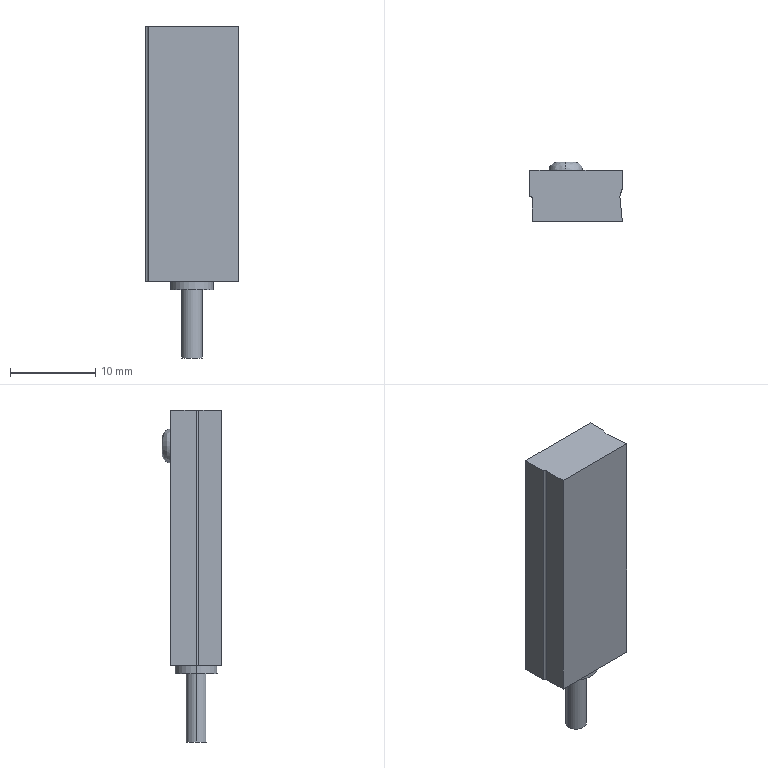Part | STEP file | HI_S-CS-95 | 1 solid | 42 faces | box 10.9 x 7 x 39 mm | volume 1983 mm3 | plane 35 | cylinder 5 | spline 2 | commonest cylinder face diameters 2.4 x2 5 x2 0.6 x1